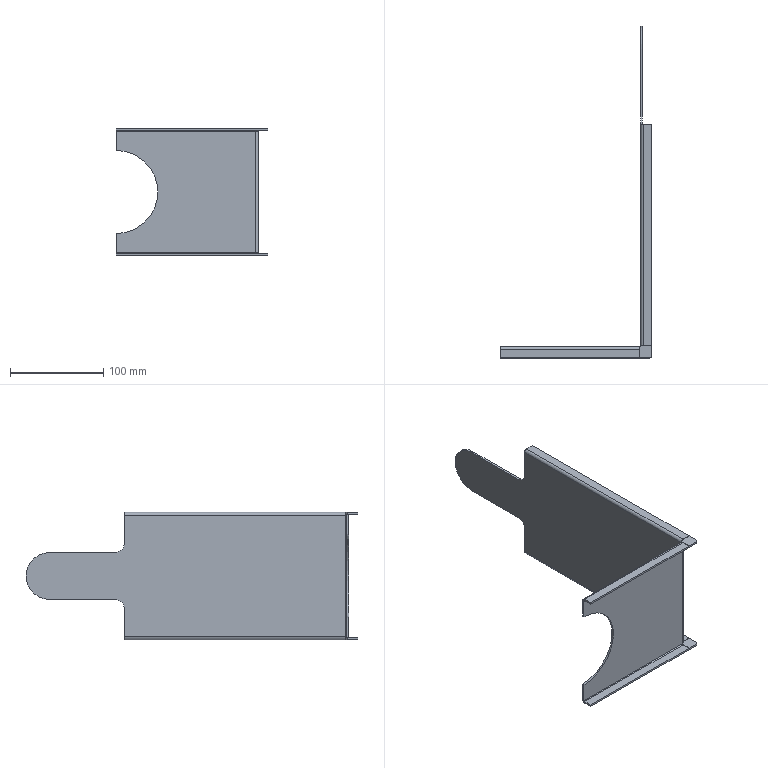Part | SolidWorks | features ICE 3, EdgeFlange 2, Fillet 1, FlatPattern 1, SMBaseFlange 1, SheetMetal 1 | 3 solids | 71 faces | box 162 x 355 x 136 mm | volume 124416 mm3 | plane 54 | cylinder 17 | commonest cylinder face diameters 2 x5 6 x5 4 x2 20 x2 50 x2 89 x1